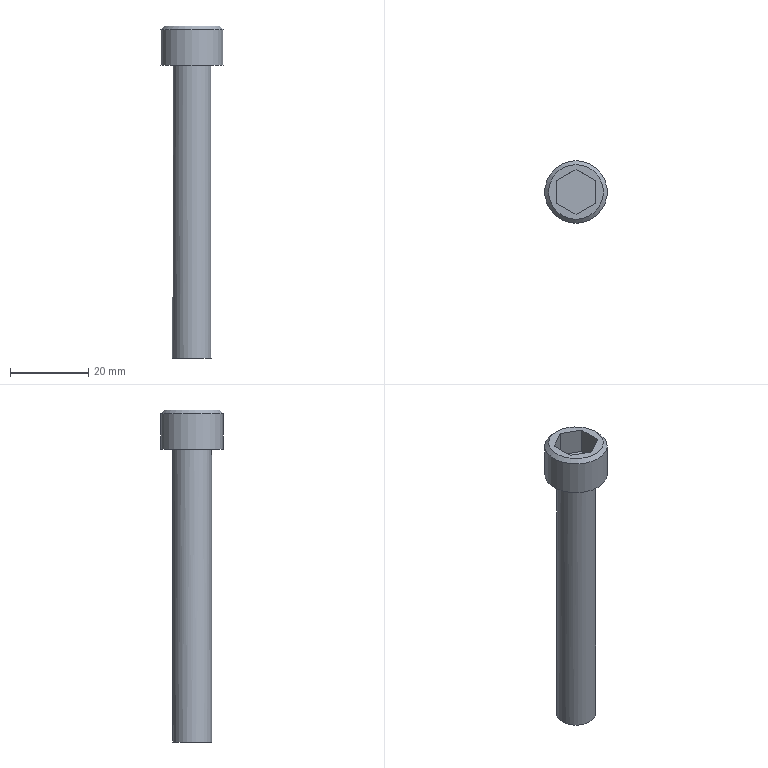Part | NX | features solid 2 | 1 solid | 13 faces | box 16 x 16 x 85 mm | volume 7300 mm3 | plane 10 | cylinder 2 | cone 1 | commonest cylinder face diameters 10 x1 16 x1
STEP:
#1=CARTESIAN_POINT('',(-1473.255,417.161,49.));
#2=VERTEX_POINT('',#1);
#3=CARTESIAN_POINT('',(-1473.255,409.161,49.));
#4=DIRECTION('',(0.,0.,1.));
#5=DIRECTION('',(0.,1.,0.));
#6=AXIS2_PLACEMENT_3D('',#3,#4,#5);
#7=CIRCLE('',#6,8.);
#8=EDGE_CURVE('',#2,#2,#7,.F.);
#9=ORIENTED_EDGE('',*,*,#8,.T.);
#10=EDGE_LOOP('',(#9));
#11=FACE_BOUND('',#10,.T.);
#12=CARTESIAN_POINT('',(-1473.255,417.161,40.));
#13=VERTEX_POINT('',#12);
#14=CARTESIAN_POINT('',(-1473.255,409.161,40.));
#15=DIRECTION('',(0.,0.,1.));
#16=DIRECTION('',(0.,1.,0.));
#17=AXIS2_PLACEMENT_3D('',#14,#15,#16);
#18=CIRCLE('',#17,8.);
#19=EDGE_CURVE('',#13,#13,#18,.T.);
#20=ORIENTED_EDGE('',*,*,#19,.T.);
#21=EDGE_LOOP('',(#20));
#22=FACE_BOUND('',#21,.T.);
#23=CARTESIAN_POINT('',(-1473.255,409.161,40.));
#24=DIRECTION('',(0.,0.,1.));
#25=DIRECTION('',(0.,1.,0.));
#26=AXIS2_PLACEMENT_3D('',#23,#24,#25);
#27=CYLINDRICAL_SURFACE('',#26,8.);
#28=ADVANCED_FACE('',(#11,#22),#27,.T.);
#29=CARTESIAN_POINT('',(-1473.255,404.161,40.));
#30=VERTEX_POINT('',#29);
#31=CARTESIAN_POINT('',(-1473.255,409.161,40.));
#32=DIRECTION('',(0.,0.,-1.));
#33=DIRECTION('',(0.,-1.,0.));
#34=AXIS2_PLACEMENT_3D('',#31,#32,#33);
#35=CIRCLE('',#34,5.);
#36=EDGE_CURVE('',#30,#30,#35,.T.);
#37=ORIENTED_EDGE('',*,*,#36,.F.);
#38=EDGE_LOOP('',(#37));
#39=FACE_BOUND('',#38,.T.);
#40=ORIENTED_EDGE('',*,*,#19,.F.);
#41=EDGE_LOOP('',(#40));
#42=FACE_BOUND('',#41,.T.);
#43=CARTESIAN_POINT('',(-1473.255,409.161,40.));
#44=DIRECTION('',(0.,0.,1.));
#45=DIRECTION('',(0.,1.,0.));
#46=AXIS2_PLACEMENT_3D('',#43,#44,#45);
#47=PLANE('',#46);
#48=ADVANCED_FACE('',(#39,#42),#47,.F.);
#49=CARTESIAN_POINT('',(-1473.255,416.161,50.));
#50=VERTEX_POINT('',#49);
#51=CARTESIAN_POINT('',(-1473.255,409.161,50.));
#52=DIRECTION('',(0.,0.,1.));
#53=DIRECTION('',(0.,1.,0.));
#54=AXIS2_PLACEMENT_3D('',#51,#52,#53);
#55=CIRCLE('',#54,7.);
#56=EDGE_CURVE('',#50,#50,#55,.T.);
#57=ORIENTED_EDGE('',*,*,#56,.T.);
#58=EDGE_LOOP('',(#57));
#59=FACE_BOUND('',#58,.T.);
#60=CARTESIAN_POINT('',(-1478.255,406.274,50.));
#61=VERTEX_POINT('',#60);
#62=CARTESIAN_POINT('',(-1473.255,403.387,50.));
#63=VERTEX_POINT('',#62);
#64=CARTESIAN_POINT('',(-1478.255,406.274,50.));
#65=DIRECTION('',(0.866,-0.5,0.));
#66=VECTOR('',#65,1000.);
#67=LINE('',#64,#66);
#68=EDGE_CURVE('',#61,#63,#67,.T.);
#69=ORIENTED_EDGE('',*,*,#68,.F.);
#70=CARTESIAN_POINT('',(-1478.255,412.047,50.));
#71=VERTEX_POINT('',#70);
#72=CARTESIAN_POINT('',(-1478.255,412.047,50.));
#73=DIRECTION('',(0.,-1.,0.));
#74=VECTOR('',#73,1000.);
#75=LINE('',#72,#74);
#76=EDGE_CURVE('',#71,#61,#75,.T.);
#77=ORIENTED_EDGE('',*,*,#76,.F.);
#78=CARTESIAN_POINT('',(-1473.255,414.934,50.));
#79=VERTEX_POINT('',#78);
#80=CARTESIAN_POINT('',(-1473.255,414.934,50.));
#81=DIRECTION('',(-0.866,-0.5,0.));
#82=VECTOR('',#81,1000.);
#83=LINE('',#80,#82);
#84=EDGE_CURVE('',#79,#71,#83,.T.);
#85=ORIENTED_EDGE('',*,*,#84,.F.);
#86=CARTESIAN_POINT('',(-1468.255,412.047,50.));
#87=VERTEX_POINT('',#86);
#88=CARTESIAN_POINT('',(-1468.255,412.047,50.));
#89=DIRECTION('',(-0.866,0.5,0.));
#90=VECTOR('',#89,1000.);
#91=LINE('',#88,#90);
#92=EDGE_CURVE('',#87,#79,#91,.T.);
#93=ORIENTED_EDGE('',*,*,#92,.F.);
#94=CARTESIAN_POINT('',(-1468.255,406.274,50.));
#95=VERTEX_POINT('',#94);
#96=CARTESIAN_POINT('',(-1468.255,406.274,50.));
#97=DIRECTION('',(0.,1.,0.));
#98=VECTOR('',#97,1000.);
#99=LINE('',#96,#98);
#100=EDGE_CURVE('',#95,#87,#99,.T.);
#101=ORIENTED_EDGE('',*,*,#100,.F.);
#102=CARTESIAN_POINT('',(-1473.255,403.387,50.));
#103=DIRECTION('',(0.866,0.5,0.));
#104=VECTOR('',#103,1000.);
#105=LINE('',#102,#104);
#106=EDGE_CURVE('',#63,#95,#105,.T.);
#107=ORIENTED_EDGE('',*,*,#106,.F.);
#108=EDGE_LOOP('',(#69,#77,#85,#93,#101,#107));
#109=FACE_BOUND('',#108,.T.);
#110=CARTESIAN_POINT('',(-1473.255,409.161,50.));
#111=DIRECTION('',(0.,0.,1.));
#112=DIRECTION('',(0.,1.,0.));
#113=AXIS2_PLACEMENT_3D('',#110,#111,#112);
#114=PLANE('',#113);
#115=ADVANCED_FACE('',(#59,#109),#114,.T.);
#116=CARTESIAN_POINT('',(-1478.255,409.161,-35.));
#117=VERTEX_POINT('',#116);
#118=CARTESIAN_POINT('',(-1473.255,409.161,-35.));
#119=DIRECTION('',(0.,0.,1.));
#120=DIRECTION('',(-1.,0.,0.));
#121=AXIS2_PLACEMENT_3D('',#118,#119,#120);
#122=CIRCLE('',#121,5.);
#123=EDGE_CURVE('',#117,#117,#122,.T.);
#124=ORIENTED_EDGE('',*,*,#123,.F.);
#125=EDGE_LOOP('',(#124));
#126=FACE_BOUND('',#125,.T.);
#127=CARTESIAN_POINT('',(-1473.255,409.161,-35.));
#128=DIRECTION('',(0.,0.,1.));
#129=DIRECTION('',(1.,0.,0.));
#130=AXIS2_PLACEMENT_3D('',#127,#128,#129);
#131=PLANE('',#130);
#132=ADVANCED_FACE('',(#126),#131,.F.);
#133=ORIENTED_EDGE('',*,*,#123,.T.);
#134=EDGE_LOOP('',(#133));
#135=FACE_BOUND('',#134,.T.);
#136=ORIENTED_EDGE('',*,*,#36,.T.);
#137=EDGE_LOOP('',(#136));
#138=FACE_BOUND('',#137,.T.);
#139=CARTESIAN_POINT('',(-1473.255,409.161,40.));
#140=DIRECTION('',(0.,0.,-1.));
#141=DIRECTION('',(0.,-1.,0.));
#142=AXIS2_PLACEMENT_3D('',#139,#140,#141);
#143=CYLINDRICAL_SURFACE('',#142,5.);
#144=ADVANCED_FACE('',(#135,#138),#143,.T.);
#145=ORIENTED_EDGE('',*,*,#68,.T.);
#146=CARTESIAN_POINT('',(-1473.255,403.387,43.333));
#147=VERTEX_POINT('',#146);
#148=CARTESIAN_POINT('',(-1473.255,403.387,43.333));
#149=DIRECTION('',(0.,0.,1.));
#150=VECTOR('',#149,1000.);
#151=LINE('',#148,#150);
#152=EDGE_CURVE('',#147,#63,#151,.T.);
#153=ORIENTED_EDGE('',*,*,#152,.F.);
#154=CARTESIAN_POINT('',(-1478.255,406.274,43.333));
#155=VERTEX_POINT('',#154);
#156=CARTESIAN_POINT('',(-1478.255,406.274,43.333));
#157=DIRECTION('',(0.866,-0.5,0.));
#158=VECTOR('',#157,1000.);
#159=LINE('',#156,#158);
#160=EDGE_CURVE('',#155,#147,#159,.T.);
#161=ORIENTED_EDGE('',*,*,#160,.F.);
#162=CARTESIAN_POINT('',(-1478.255,406.274,43.333));
#163=DIRECTION('',(0.,0.,1.));
#164=VECTOR('',#163,1000.);
#165=LINE('',#162,#164);
#166=EDGE_CURVE('',#155,#61,#165,.T.);
#167=ORIENTED_EDGE('',*,*,#166,.T.);
#168=EDGE_LOOP('',(#145,#153,#161,#167));
#169=FACE_BOUND('',#168,.T.);
#170=CARTESIAN_POINT('',(-1478.255,406.274,43.333));
#171=DIRECTION('',(-0.5,-0.866,0.));
#172=DIRECTION('',(0.866,-0.5,0.));
#173=AXIS2_PLACEMENT_3D('',#170,#171,#172);
#174=PLANE('',#173);
#175=ADVANCED_FACE('',(#169),#174,.F.);
#176=ORIENTED_EDGE('',*,*,#106,.T.);
#177=CARTESIAN_POINT('',(-1468.255,406.274,43.333));
#178=VERTEX_POINT('',#177);
#179=CARTESIAN_POINT('',(-1468.255,406.274,43.333));
#180=DIRECTION('',(0.,0.,1.));
#181=VECTOR('',#180,1000.);
#182=LINE('',#179,#181);
#183=EDGE_CURVE('',#178,#95,#182,.T.);
#184=ORIENTED_EDGE('',*,*,#183,.F.);
#185=CARTESIAN_POINT('',(-1473.255,403.387,43.333));
#186=DIRECTION('',(0.866,0.5,0.));
#187=VECTOR('',#186,1000.);
#188=LINE('',#185,#187);
#189=EDGE_CURVE('',#147,#178,#188,.T.);
#190=ORIENTED_EDGE('',*,*,#189,.F.);
#191=ORIENTED_EDGE('',*,*,#152,.T.);
#192=EDGE_LOOP('',(#176,#184,#190,#191));
#193=FACE_BOUND('',#192,.T.);
#194=CARTESIAN_POINT('',(-1473.255,403.387,43.333));
#195=DIRECTION('',(0.5,-0.866,0.));
#196=DIRECTION('',(0.866,0.5,0.));
#197=AXIS2_PLACEMENT_3D('',#194,#195,#196);
#198=PLANE('',#197);
#199=ADVANCED_FACE('',(#193),#198,.F.);
#200=ORIENTED_EDGE('',*,*,#100,.T.);
#201=CARTESIAN_POINT('',(-1468.255,412.047,43.333));
#202=VERTEX_POINT('',#201);
#203=CARTESIAN_POINT('',(-1468.255,412.047,43.333));
#204=DIRECTION('',(0.,0.,1.));
#205=VECTOR('',#204,1000.);
#206=LINE('',#203,#205);
#207=EDGE_CURVE('',#202,#87,#206,.T.);
#208=ORIENTED_EDGE('',*,*,#207,.F.);
#209=CARTESIAN_POINT('',(-1468.255,406.274,43.333));
#210=DIRECTION('',(0.,1.,0.));
#211=VECTOR('',#210,1000.);
#212=LINE('',#209,#211);
#213=EDGE_CURVE('',#178,#202,#212,.T.);
#214=ORIENTED_EDGE('',*,*,#213,.F.);
#215=ORIENTED_EDGE('',*,*,#183,.T.);
#216=EDGE_LOOP('',(#200,#208,#214,#215));
#217=FACE_BOUND('',#216,.T.);
#218=CARTESIAN_POINT('',(-1468.255,406.274,43.333));
#219=DIRECTION('',(1.,0.,0.));
#220=DIRECTION('',(0.,0.,-1.));
#221=AXIS2_PLACEMENT_3D('',#218,#219,#220);
#222=PLANE('',#221);
#223=ADVANCED_FACE('',(#217),#222,.F.);
#224=ORIENTED_EDGE('',*,*,#92,.T.);
#225=CARTESIAN_POINT('',(-1473.255,414.934,43.333));
#226=VERTEX_POINT('',#225);
#227=CARTESIAN_POINT('',(-1473.255,414.934,43.333));
#228=DIRECTION('',(0.,0.,1.));
#229=VECTOR('',#228,1000.);
#230=LINE('',#227,#229);
#231=EDGE_CURVE('',#226,#79,#230,.T.);
#232=ORIENTED_EDGE('',*,*,#231,.F.);
#233=CARTESIAN_POINT('',(-1468.255,412.047,43.333));
#234=DIRECTION('',(-0.866,0.5,0.));
#235=VECTOR('',#234,1000.);
#236=LINE('',#233,#235);
#237=EDGE_CURVE('',#202,#226,#236,.T.);
#238=ORIENTED_EDGE('',*,*,#237,.F.);
#239=ORIENTED_EDGE('',*,*,#207,.T.);
#240=EDGE_LOOP('',(#224,#232,#238,#239));
#241=FACE_BOUND('',#240,.T.);
#242=CARTESIAN_POINT('',(-1468.255,412.047,43.333));
#243=DIRECTION('',(0.5,0.866,0.));
#244=DIRECTION('',(-0.866,0.5,0.));
#245=AXIS2_PLACEMENT_3D('',#242,#243,#244);
#246=PLANE('',#245);
#247=ADVANCED_FACE('',(#241),#246,.F.);
#248=ORIENTED_EDGE('',*,*,#84,.T.);
#249=CARTESIAN_POINT('',(-1478.255,412.047,43.333));
#250=VERTEX_POINT('',#249);
#251=CARTESIAN_POINT('',(-1478.255,412.047,43.333));
#252=DIRECTION('',(0.,0.,1.));
#253=VECTOR('',#252,1000.);
#254=LINE('',#251,#253);
#255=EDGE_CURVE('',#250,#71,#254,.T.);
#256=ORIENTED_EDGE('',*,*,#255,.F.);
#257=CARTESIAN_POINT('',(-1473.255,414.934,43.333));
#258=DIRECTION('',(-0.866,-0.5,0.));
#259=VECTOR('',#258,1000.);
#260=LINE('',#257,#259);
#261=EDGE_CURVE('',#226,#250,#260,.T.);
#262=ORIENTED_EDGE('',*,*,#261,.F.);
#263=ORIENTED_EDGE('',*,*,#231,.T.);
#264=EDGE_LOOP('',(#248,#256,#262,#263));
#265=FACE_BOUND('',#264,.T.);
#266=CARTESIAN_POINT('',(-1473.255,414.934,43.333));
#267=DIRECTION('',(-0.5,0.866,0.));
#268=DIRECTION('',(-0.866,-0.5,0.));
#269=AXIS2_PLACEMENT_3D('',#266,#267,#268);
#270=PLANE('',#269);
#271=ADVANCED_FACE('',(#265),#270,.F.);
#272=ORIENTED_EDGE('',*,*,#76,.T.);
#273=ORIENTED_EDGE('',*,*,#166,.F.);
#274=CARTESIAN_POINT('',(-1478.255,412.047,43.333));
#275=DIRECTION('',(0.,-1.,0.));
#276=VECTOR('',#275,1000.);
#277=LINE('',#274,#276);
#278=EDGE_CURVE('',#250,#155,#277,.T.);
#279=ORIENTED_EDGE('',*,*,#278,.F.);
#280=ORIENTED_EDGE('',*,*,#255,.T.);
#281=EDGE_LOOP('',(#272,#273,#279,#280));
#282=FACE_BOUND('',#281,.T.);
#283=CARTESIAN_POINT('',(-1478.255,412.047,43.333));
#284=DIRECTION('',(-1.,0.,0.));
#285=DIRECTION('',(0.,-1.,0.));
#286=AXIS2_PLACEMENT_3D('',#283,#284,#285);
#287=PLANE('',#286);
#288=ADVANCED_FACE('',(#282),#287,.F.);
#289=ORIENTED_EDGE('',*,*,#160,.T.);
#290=ORIENTED_EDGE('',*,*,#189,.T.);
#291=ORIENTED_EDGE('',*,*,#213,.T.);
#292=ORIENTED_EDGE('',*,*,#237,.T.);
#293=ORIENTED_EDGE('',*,*,#261,.T.);
#294=ORIENTED_EDGE('',*,*,#278,.T.);
#295=EDGE_LOOP('',(#289,#290,#291,#292,#293,#294));
#296=FACE_BOUND('',#295,.T.);
#297=CARTESIAN_POINT('',(-1473.255,403.387,43.333));
#298=DIRECTION('',(0.,0.,1.));
#299=DIRECTION('',(0.,1.,0.));
#300=AXIS2_PLACEMENT_3D('',#297,#298,#299);
#301=PLANE('',#300);
#302=ADVANCED_FACE('',(#296),#301,.T.);
#303=ORIENTED_EDGE('',*,*,#8,.F.);
#304=EDGE_LOOP('',(#303));
#305=FACE_BOUND('',#304,.T.);
#306=ORIENTED_EDGE('',*,*,#56,.F.);
#307=EDGE_LOOP('',(#306));
#308=FACE_BOUND('',#307,.T.);
#309=CARTESIAN_POINT('',(-1473.255,409.161,50.));
#310=DIRECTION('',(0.,0.,-1.));
#311=DIRECTION('',(0.,-1.,0.));
#312=AXIS2_PLACEMENT_3D('',#309,#310,#311);
#313=CONICAL_SURFACE('',#312,7.,0.7854);
#314=ADVANCED_FACE('',(#305,#308),#313,.T.);
#315=CLOSED_SHELL('',(#28,#48,#115,#132,#144,#175,#199,#223,#247,#271,#288,#302,#314));
#316=MANIFOLD_SOLID_BREP('',#315);
#317=(LENGTH_UNIT()NAMED_UNIT(*)SI_UNIT(.MILLI.,.METRE.));
#318=UNCERTAINTY_MEASURE_WITH_UNIT(LENGTH_MEASURE(0.00001),#317,'','');
#319=(NAMED_UNIT(*)PLANE_ANGLE_UNIT()SI_UNIT($,.RADIAN.));
#320=(NAMED_UNIT(*)SI_UNIT($,.STERADIAN.)SOLID_ANGLE_UNIT());
#321=(GEOMETRIC_REPRESENTATION_CONTEXT(3)GLOBAL_UNCERTAINTY_ASSIGNED_CONTEXT((#318))GLOBAL_UNIT_ASSIGNED_CONTEXT((#317,#319,#320))REPRESENTATION_CONTEXT('',''));
#322=ADVANCED_BREP_SHAPE_REPRESENTATION('',(#316),#321);